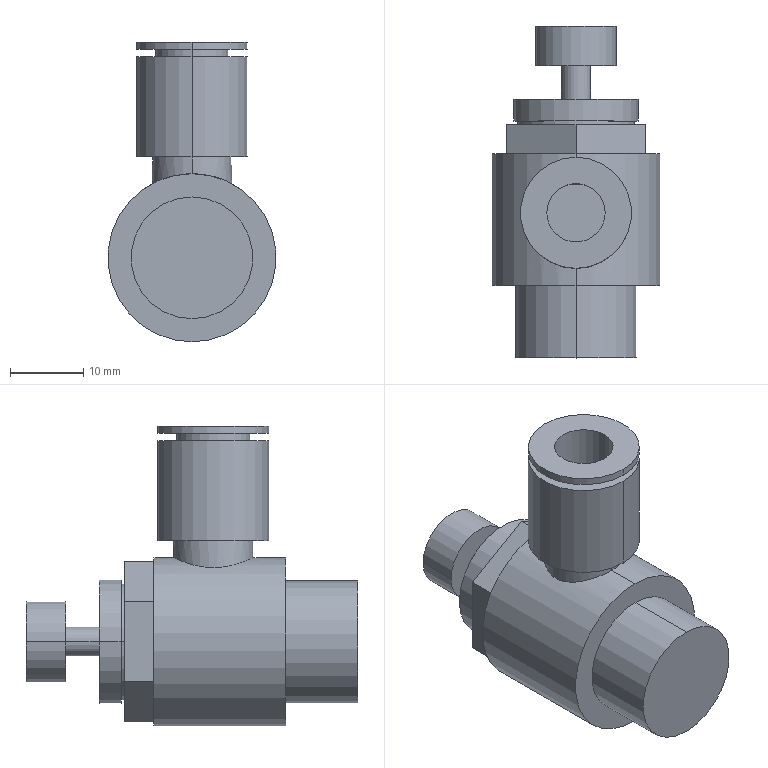Part | STEP file | Speed control valve AS3201F-03-08SA | 1 solid | 41 faces | box 23 x 45.4 x 41 mm | volume 14301 mm3 | cylinder 22 | plane 19 | commonest cylinder face diameters 15.2 x4 4 x2 8 x2 10 x2 10.88 x2 11 x2